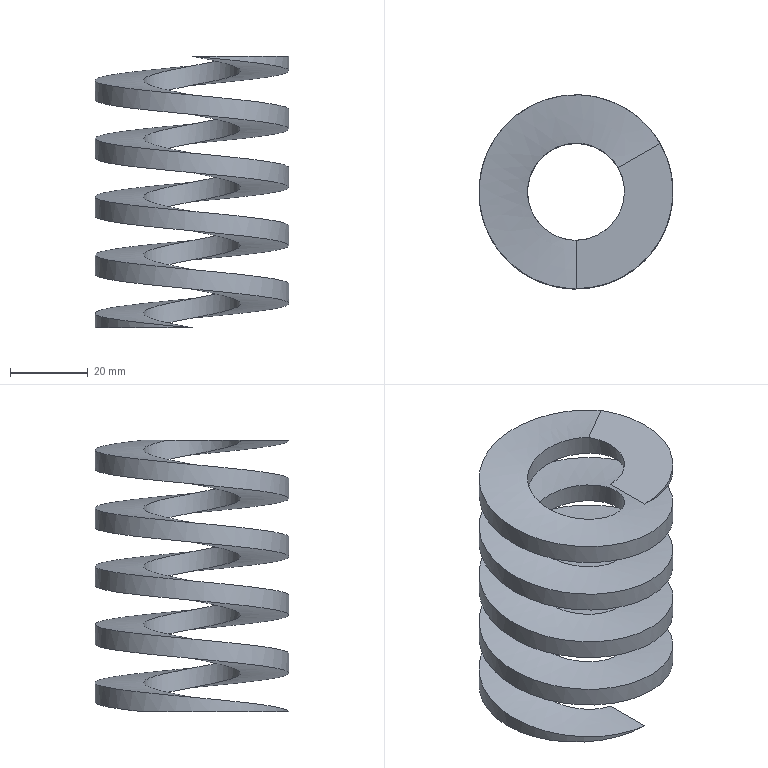Part | NX | features solid 2 | 1 solid | 6 faces | box 50 x 50 x 70 mm | volume 34357 mm3 | plane 2 | spline 2 | cylinder 2 | commonest cylinder face diameters 25 x1 50 x1